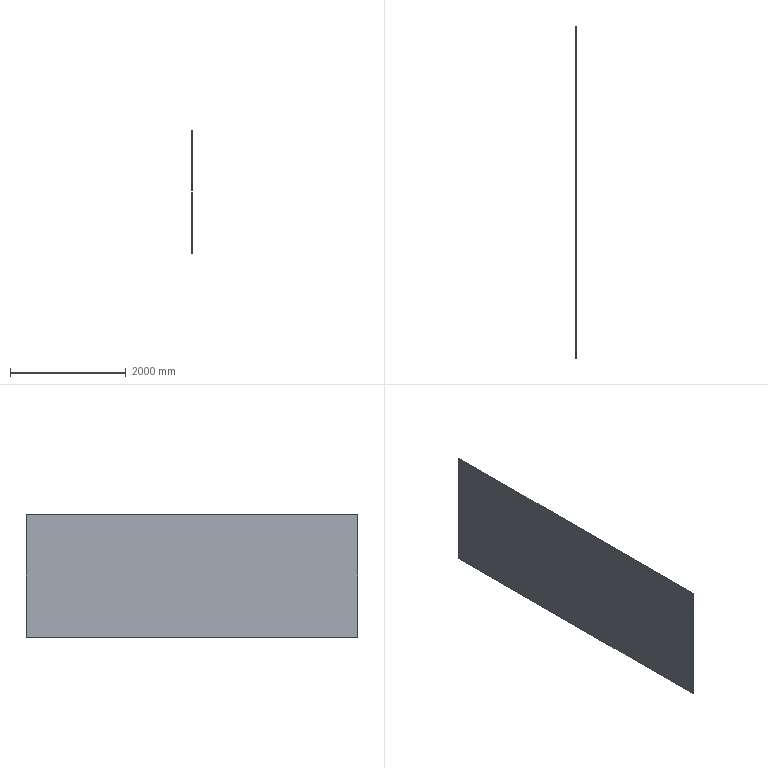Part | SolidWorks | features Extrusion 1 | 1 solid | 6 faces | box 5 x 5744 x 2124 mm | volume 61001280 mm3 | plane 6
STEP:
#1=CARTESIAN_POINT('',(-95.,-2872.,1062.));
#2=VERTEX_POINT('',#1);
#3=CARTESIAN_POINT('',(-95.,2872.,1062.));
#4=VERTEX_POINT('',#3);
#5=CARTESIAN_POINT('',(-95.,-2872.,1062.));
#6=DIRECTION('',(0.,1.,0.));
#7=VECTOR('',#6,1000.);
#8=LINE('',#5,#7);
#9=EDGE_CURVE('',#2,#4,#8,.T.);
#10=ORIENTED_EDGE('',*,*,#9,.T.);
#11=CARTESIAN_POINT('',(-100.,2872.,1062.));
#12=VERTEX_POINT('',#11);
#13=CARTESIAN_POINT('',(-100.,2872.,1062.));
#14=DIRECTION('',(1.,0.,0.));
#15=VECTOR('',#14,1000.);
#16=LINE('',#13,#15);
#17=EDGE_CURVE('',#12,#4,#16,.T.);
#18=ORIENTED_EDGE('',*,*,#17,.F.);
#19=CARTESIAN_POINT('',(-100.,-2872.,1062.));
#20=VERTEX_POINT('',#19);
#21=CARTESIAN_POINT('',(-100.,-2872.,1062.));
#22=DIRECTION('',(0.,1.,0.));
#23=VECTOR('',#22,1000.);
#24=LINE('',#21,#23);
#25=EDGE_CURVE('',#20,#12,#24,.T.);
#26=ORIENTED_EDGE('',*,*,#25,.F.);
#27=CARTESIAN_POINT('',(-100.,-2872.,1062.));
#28=DIRECTION('',(1.,0.,0.));
#29=VECTOR('',#28,1000.);
#30=LINE('',#27,#29);
#31=EDGE_CURVE('',#20,#2,#30,.T.);
#32=ORIENTED_EDGE('',*,*,#31,.T.);
#33=EDGE_LOOP('',(#10,#18,#26,#32));
#34=FACE_OUTER_BOUND('',#33,.T.);
#35=CARTESIAN_POINT('',(-100.,-2872.,1062.));
#36=DIRECTION('',(0.,0.,-1.));
#37=DIRECTION('',(-1.,0.,0.));
#38=AXIS2_PLACEMENT_3D('',#35,#36,#37);
#39=PLANE('',#38);
#40=ADVANCED_FACE('',(#34),#39,.F.);
#41=CARTESIAN_POINT('',(-95.,2872.,-1062.));
#42=VERTEX_POINT('',#41);
#43=CARTESIAN_POINT('',(-95.,2872.,-1062.));
#44=DIRECTION('',(0.,0.,-1.));
#45=VECTOR('',#44,1000.);
#46=LINE('',#43,#45);
#47=EDGE_CURVE('',#4,#42,#46,.T.);
#48=ORIENTED_EDGE('',*,*,#47,.T.);
#49=CARTESIAN_POINT('',(-100.,2872.,-1062.));
#50=VERTEX_POINT('',#49);
#51=CARTESIAN_POINT('',(-100.,2872.,-1062.));
#52=DIRECTION('',(1.,0.,0.));
#53=VECTOR('',#52,1000.);
#54=LINE('',#51,#53);
#55=EDGE_CURVE('',#50,#42,#54,.T.);
#56=ORIENTED_EDGE('',*,*,#55,.F.);
#57=CARTESIAN_POINT('',(-100.,2872.,-1062.));
#58=DIRECTION('',(0.,0.,-1.));
#59=VECTOR('',#58,1000.);
#60=LINE('',#57,#59);
#61=EDGE_CURVE('',#12,#50,#60,.T.);
#62=ORIENTED_EDGE('',*,*,#61,.F.);
#63=ORIENTED_EDGE('',*,*,#17,.T.);
#64=EDGE_LOOP('',(#48,#56,#62,#63));
#65=FACE_OUTER_BOUND('',#64,.T.);
#66=CARTESIAN_POINT('',(-100.,2872.,-1062.));
#67=DIRECTION('',(0.,-1.,0.));
#68=DIRECTION('',(1.,0.,0.));
#69=AXIS2_PLACEMENT_3D('',#66,#67,#68);
#70=PLANE('',#69);
#71=ADVANCED_FACE('',(#65),#70,.F.);
#72=CARTESIAN_POINT('',(-95.,-2872.,-1062.));
#73=VERTEX_POINT('',#72);
#74=CARTESIAN_POINT('',(-95.,-2872.,-1062.));
#75=DIRECTION('',(0.,-1.,0.));
#76=VECTOR('',#75,1000.);
#77=LINE('',#74,#76);
#78=EDGE_CURVE('',#42,#73,#77,.T.);
#79=ORIENTED_EDGE('',*,*,#78,.T.);
#80=CARTESIAN_POINT('',(-100.,-2872.,-1062.));
#81=VERTEX_POINT('',#80);
#82=CARTESIAN_POINT('',(-100.,-2872.,-1062.));
#83=DIRECTION('',(1.,0.,0.));
#84=VECTOR('',#83,1000.);
#85=LINE('',#82,#84);
#86=EDGE_CURVE('',#81,#73,#85,.T.);
#87=ORIENTED_EDGE('',*,*,#86,.F.);
#88=CARTESIAN_POINT('',(-100.,-2872.,-1062.));
#89=DIRECTION('',(0.,-1.,0.));
#90=VECTOR('',#89,1000.);
#91=LINE('',#88,#90);
#92=EDGE_CURVE('',#50,#81,#91,.T.);
#93=ORIENTED_EDGE('',*,*,#92,.F.);
#94=ORIENTED_EDGE('',*,*,#55,.T.);
#95=EDGE_LOOP('',(#79,#87,#93,#94));
#96=FACE_OUTER_BOUND('',#95,.T.);
#97=CARTESIAN_POINT('',(-100.,-2872.,-1062.));
#98=DIRECTION('',(0.,0.,1.));
#99=DIRECTION('',(1.,0.,0.));
#100=AXIS2_PLACEMENT_3D('',#97,#98,#99);
#101=PLANE('',#100);
#102=ADVANCED_FACE('',(#96),#101,.F.);
#103=CARTESIAN_POINT('',(-95.,-2872.,-1062.));
#104=DIRECTION('',(0.,0.,1.));
#105=VECTOR('',#104,1000.);
#106=LINE('',#103,#105);
#107=EDGE_CURVE('',#73,#2,#106,.T.);
#108=ORIENTED_EDGE('',*,*,#107,.T.);
#109=ORIENTED_EDGE('',*,*,#31,.F.);
#110=CARTESIAN_POINT('',(-100.,-2872.,-1062.));
#111=DIRECTION('',(0.,0.,1.));
#112=VECTOR('',#111,1000.);
#113=LINE('',#110,#112);
#114=EDGE_CURVE('',#81,#20,#113,.T.);
#115=ORIENTED_EDGE('',*,*,#114,.F.);
#116=ORIENTED_EDGE('',*,*,#86,.T.);
#117=EDGE_LOOP('',(#108,#109,#115,#116));
#118=FACE_OUTER_BOUND('',#117,.T.);
#119=CARTESIAN_POINT('',(-100.,-2872.,-1062.));
#120=DIRECTION('',(0.,1.,0.));
#121=DIRECTION('',(-1.,0.,0.));
#122=AXIS2_PLACEMENT_3D('',#119,#120,#121);
#123=PLANE('',#122);
#124=ADVANCED_FACE('',(#118),#123,.F.);
#125=ORIENTED_EDGE('',*,*,#25,.T.);
#126=ORIENTED_EDGE('',*,*,#61,.T.);
#127=ORIENTED_EDGE('',*,*,#92,.T.);
#128=ORIENTED_EDGE('',*,*,#114,.T.);
#129=EDGE_LOOP('',(#125,#126,#127,#128));
#130=FACE_OUTER_BOUND('',#129,.T.);
#131=CARTESIAN_POINT('',(-100.,0.,0.));
#132=DIRECTION('',(1.,0.,0.));
#133=DIRECTION('',(0.,1.,0.));
#134=AXIS2_PLACEMENT_3D('',#131,#132,#133);
#135=PLANE('',#134);
#136=ADVANCED_FACE('',(#130),#135,.F.);
#137=ORIENTED_EDGE('',*,*,#9,.F.);
#138=ORIENTED_EDGE('',*,*,#107,.F.);
#139=ORIENTED_EDGE('',*,*,#78,.F.);
#140=ORIENTED_EDGE('',*,*,#47,.F.);
#141=EDGE_LOOP('',(#137,#138,#139,#140));
#142=FACE_OUTER_BOUND('',#141,.T.);
#143=CARTESIAN_POINT('',(-95.,0.,0.));
#144=DIRECTION('',(1.,0.,0.));
#145=DIRECTION('',(0.,1.,0.));
#146=AXIS2_PLACEMENT_3D('',#143,#144,#145);
#147=PLANE('',#146);
#148=ADVANCED_FACE('',(#142),#147,.T.);
#149=CLOSED_SHELL('',(#40,#71,#102,#124,#136,#148));
#150=MANIFOLD_SOLID_BREP('',#149);
#151=CARTESIAN_POINT('',(0.,0.,0.));
#152=DIRECTION('',(0.,0.,1.));
#153=DIRECTION('',(1.,0.,0.));
#154=AXIS2_PLACEMENT_3D('',#151,#152,#153);
#155=(LENGTH_UNIT()NAMED_UNIT(*)SI_UNIT(.MILLI.,.METRE.));
#156=UNCERTAINTY_MEASURE_WITH_UNIT(LENGTH_MEASURE(0.00001),#155,'','');
#157=(NAMED_UNIT(*)PLANE_ANGLE_UNIT()SI_UNIT($,.RADIAN.));
#158=(NAMED_UNIT(*)SI_UNIT($,.STERADIAN.)SOLID_ANGLE_UNIT());
#159=(GEOMETRIC_REPRESENTATION_CONTEXT(3)GLOBAL_UNCERTAINTY_ASSIGNED_CONTEXT((#156))GLOBAL_UNIT_ASSIGNED_CONTEXT((#155,#157,#158))REPRESENTATION_CONTEXT('',''));
#160=ADVANCED_BREP_SHAPE_REPRESENTATION('',(#150,#154),#159);